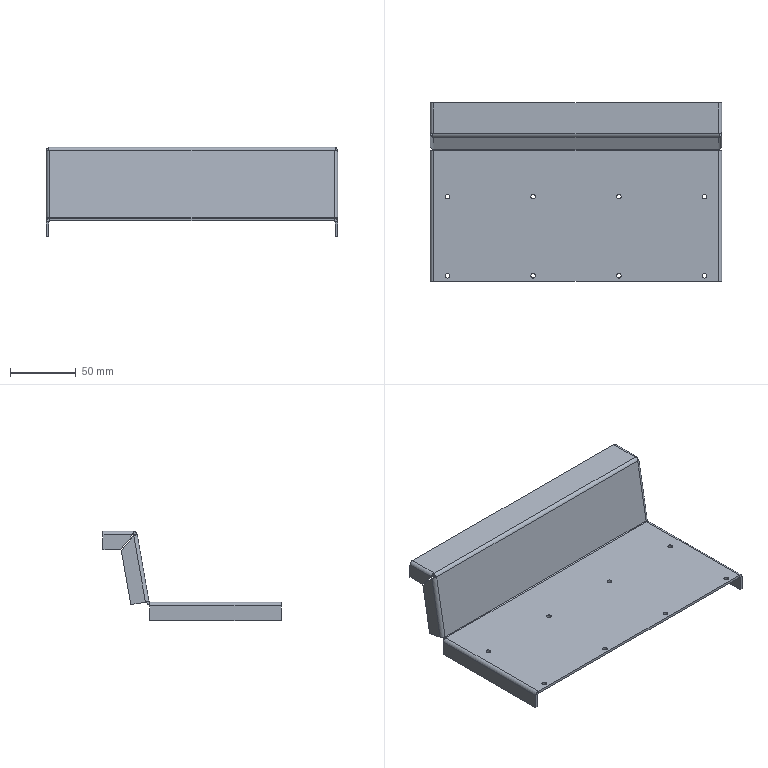Part | STEP file | Screw feeder-hopper inclined plate_default | 1 solid | 94 faces | box 221 x 135.003 x 67.848 mm | volume 86374 mm3 | plane 58 | cylinder 32 | spline 4 | commonest cylinder face diameters 3.5 x16 1.473 x8 5.473 x8